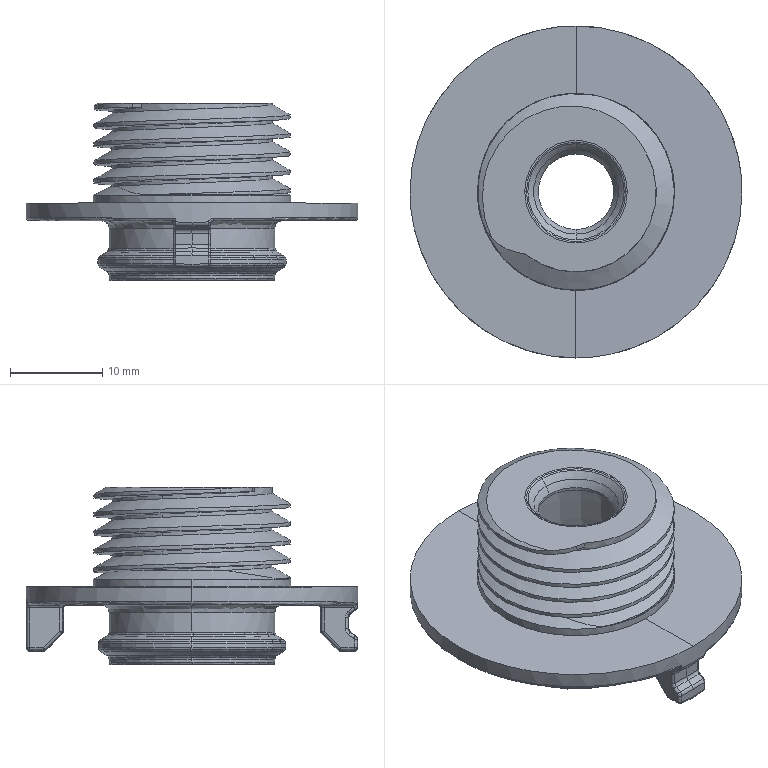Part | STEP file | ZXCOMPANY_A722-L-150 | 1 solid | 194 faces | box 36 x 36 x 19.3 mm | volume 4496 mm3 | cylinder 65 | torus 42 | spline 32 | plane 29 | cone 14 | sphere 12 | commonest cylinder face diameters 0.6 x39 17.4 x9 1 x4 18 x4 36 x3 8.187 x2